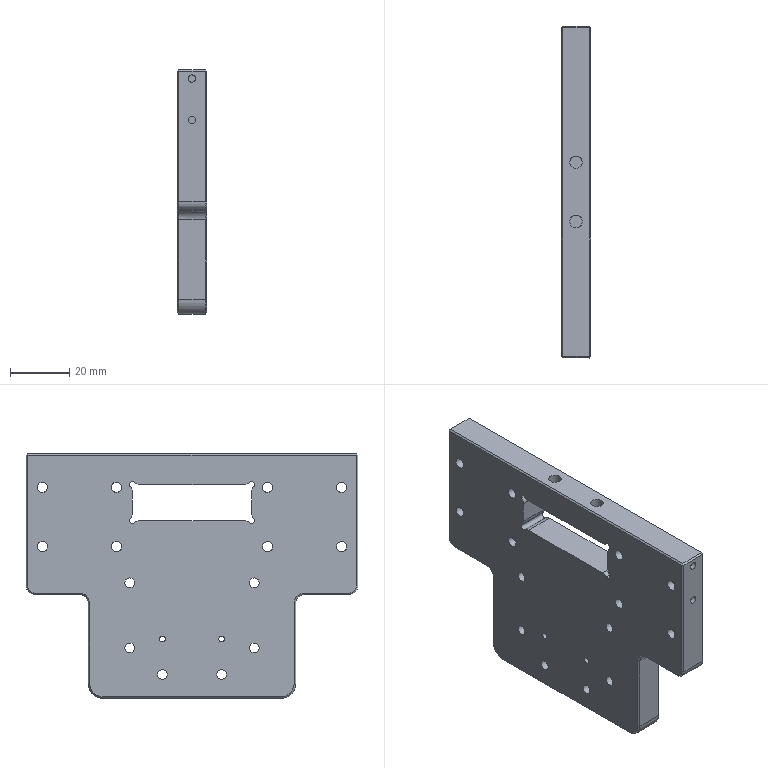Part | 1 solid | 120 faces | box 10 x 112 x 82.562 mm | volume 69469 mm3 | cylinder 50 | plane 48 | cone 22 | commonest cylinder face diameters 6 x12 3.5 x8 5 x8 2 x6 3.3 x6 2.5 x4